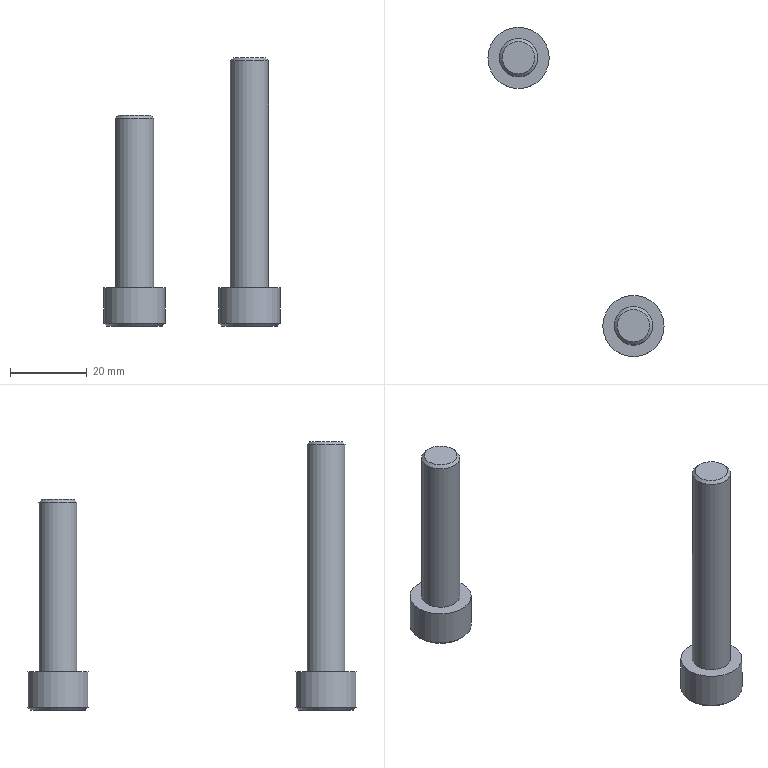Part | STEP file | M10.00-45 | 2 solids | 28 faces | box 46 x 86 x 70 mm | volume 11598 mm3 | plane 20 | cylinder 4 | cone 4 | commonest cylinder face diameters 10 x2 16 x2